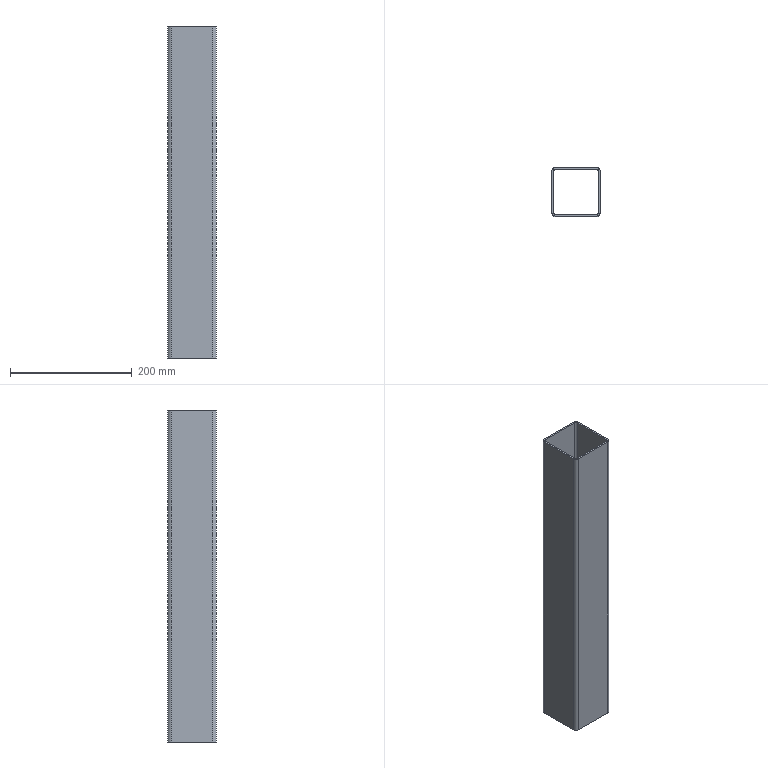Part | STEP file | SN10_008_006-01_TUBO_QUADRADO | 1 solid | 18 faces | box 80 x 80 x 546 mm | volume 491849 mm3 | plane 10 | cylinder 8 | commonest cylinder face diameters 6 x4 12 x4
STEP:
#1=CARTESIAN_POINT('',(0.,0.,0.));
#2=DIRECTION('',(0.,0.,1.));
#3=DIRECTION('',(1.,0.,0.));
#4=AXIS2_PLACEMENT_3D('',#1,#2,#3);
#5=CARTESIAN_POINT('',(323.629,344.,446.));
#6=VERTEX_POINT('',#5);
#7=CARTESIAN_POINT('',(323.629,276.,446.));
#8=VERTEX_POINT('',#7);
#9=CARTESIAN_POINT('',(323.629,344.,446.));
#10=DIRECTION('',(0.,-1.,0.));
#11=VECTOR('',#10,1.);
#12=LINE('',#9,#11);
#13=CARTESIAN_POINT('',(323.629,344.,-115.));
#14=DIRECTION('',(-1.,0.,0.));
#15=DIRECTION('',(0.,0.,1.));
#16=AXIS2_PLACEMENT_3D('',#13,#14,#15);
#17=PLANE('',#16);
#18=CARTESIAN_POINT('',(561.,0.));
#19=DIRECTION('',(0.,-1.));
#20=VECTOR('',#19,1.);
#21=LINE('',#18,#20);
#22=(GEOMETRIC_REPRESENTATION_CONTEXT(2)PARAMETRIC_REPRESENTATION_CONTEXT()REPRESENTATION_CONTEXT('',''));
#23=DEFINITIONAL_REPRESENTATION('',(#21),#22);
#24=PCURVE('',#17,#23);
#25=CARTESIAN_POINT('',(323.629,250.,446.));
#26=DIRECTION('',(0.,0.,-1.));
#27=DIRECTION('',(-1.,0.,0.));
#28=AXIS2_PLACEMENT_3D('',#25,#26,#27);
#29=PLANE('',#28);
#30=CARTESIAN_POINT('',(0.,94.));
#31=DIRECTION('',(0.,-1.));
#32=VECTOR('',#31,1.);
#33=LINE('',#30,#32);
#34=(GEOMETRIC_REPRESENTATION_CONTEXT(2)PARAMETRIC_REPRESENTATION_CONTEXT()REPRESENTATION_CONTEXT('',''));
#35=DEFINITIONAL_REPRESENTATION('',(#33),#34);
#36=PCURVE('',#29,#35);
#37=SURFACE_CURVE('',#12,(#24,#36),.PCURVE_S1.);
#38=EDGE_CURVE('',#6,#8,#37,.T.);
#39=ORIENTED_EDGE('',*,*,#38,.T.);
#40=CARTESIAN_POINT('',(323.629,276.,-100.));
#41=VERTEX_POINT('',#40);
#42=CARTESIAN_POINT('',(323.629,276.,446.));
#43=DIRECTION('',(0.,0.,-1.));
#44=VECTOR('',#43,1.);
#45=LINE('',#42,#44);
#46=CARTESIAN_POINT('',(561.,-68.));
#47=DIRECTION('',(-1.,0.));
#48=VECTOR('',#47,1.);
#49=LINE('',#46,#48);
#50=(GEOMETRIC_REPRESENTATION_CONTEXT(2)PARAMETRIC_REPRESENTATION_CONTEXT()REPRESENTATION_CONTEXT('',''));
#51=DEFINITIONAL_REPRESENTATION('',(#49),#50);
#52=PCURVE('',#17,#51);
#53=CARTESIAN_POINT('',(317.629,276.,176.11));
#54=DIRECTION('',(0.,0.,1.));
#55=DIRECTION('',(0.,-1.,0.));
#56=AXIS2_PLACEMENT_3D('',#53,#54,#55);
#57=CYLINDRICAL_SURFACE('',#56,6.);
#58=CARTESIAN_POINT('',(1.571,269.89));
#59=DIRECTION('',(0.,-1.));
#60=VECTOR('',#59,1.);
#61=LINE('',#58,#60);
#62=(GEOMETRIC_REPRESENTATION_CONTEXT(2)PARAMETRIC_REPRESENTATION_CONTEXT()REPRESENTATION_CONTEXT('',''));
#63=DEFINITIONAL_REPRESENTATION('',(#61),#62);
#64=PCURVE('',#57,#63);
#65=SURFACE_CURVE('',#45,(#52,#64),.PCURVE_S1.);
#66=EDGE_CURVE('',#8,#41,#65,.T.);
#67=ORIENTED_EDGE('',*,*,#66,.T.);
#68=CARTESIAN_POINT('',(323.629,344.,-100.));
#69=VERTEX_POINT('',#68);
#70=CARTESIAN_POINT('',(323.629,344.,-100.));
#71=DIRECTION('',(0.,-1.,0.));
#72=VECTOR('',#71,1.);
#73=LINE('',#70,#72);
#74=CARTESIAN_POINT('',(15.,0.));
#75=DIRECTION('',(0.,-1.));
#76=VECTOR('',#75,1.);
#77=LINE('',#74,#76);
#78=(GEOMETRIC_REPRESENTATION_CONTEXT(2)PARAMETRIC_REPRESENTATION_CONTEXT()REPRESENTATION_CONTEXT('',''));
#79=DEFINITIONAL_REPRESENTATION('',(#77),#78);
#80=PCURVE('',#17,#79);
#81=CARTESIAN_POINT('',(0.,0.,-100.));
#82=DIRECTION('',(0.,0.,1.));
#83=DIRECTION('',(1.,0.,0.));
#84=AXIS2_PLACEMENT_3D('',#81,#82,#83);
#85=PLANE('',#84);
#86=CARTESIAN_POINT('',(323.629,344.));
#87=DIRECTION('',(0.,-1.));
#88=VECTOR('',#87,1.);
#89=LINE('',#86,#88);
#90=(GEOMETRIC_REPRESENTATION_CONTEXT(2)PARAMETRIC_REPRESENTATION_CONTEXT()REPRESENTATION_CONTEXT('',''));
#91=DEFINITIONAL_REPRESENTATION('',(#89),#90);
#92=PCURVE('',#85,#91);
#93=SURFACE_CURVE('',#73,(#80,#92),.PCURVE_S1.);
#94=EDGE_CURVE('',#69,#41,#93,.T.);
#95=ORIENTED_EDGE('',*,*,#94,.F.);
#96=CARTESIAN_POINT('',(323.629,344.,446.));
#97=DIRECTION('',(0.,0.,-1.));
#98=VECTOR('',#97,1.);
#99=LINE('',#96,#98);
#100=CARTESIAN_POINT('',(561.,0.));
#101=DIRECTION('',(-1.,0.));
#102=VECTOR('',#101,1.);
#103=LINE('',#100,#102);
#104=(GEOMETRIC_REPRESENTATION_CONTEXT(2)PARAMETRIC_REPRESENTATION_CONTEXT()REPRESENTATION_CONTEXT('',''));
#105=DEFINITIONAL_REPRESENTATION('',(#103),#104);
#106=PCURVE('',#17,#105);
#107=CARTESIAN_POINT('',(317.629,344.,176.11));
#108=DIRECTION('',(0.,0.,1.));
#109=DIRECTION('',(1.,0.,0.));
#110=AXIS2_PLACEMENT_3D('',#107,#108,#109);
#111=CYLINDRICAL_SURFACE('',#110,6.);
#112=CARTESIAN_POINT('',(0.,269.89));
#113=DIRECTION('',(0.,-1.));
#114=VECTOR('',#113,1.);
#115=LINE('',#112,#114);
#116=(GEOMETRIC_REPRESENTATION_CONTEXT(2)PARAMETRIC_REPRESENTATION_CONTEXT()REPRESENTATION_CONTEXT('',''));
#117=DEFINITIONAL_REPRESENTATION('',(#115),#116);
#118=PCURVE('',#111,#117);
#119=SURFACE_CURVE('',#99,(#106,#118),.PCURVE_S1.);
#120=EDGE_CURVE('',#6,#69,#119,.T.);
#121=ORIENTED_EDGE('',*,*,#120,.F.);
#122=EDGE_LOOP('',(#39,#67,#95,#121));
#123=FACE_BOUND('',#122,.T.);
#124=ADVANCED_FACE('',(#123),#17,.F.);
#125=CARTESIAN_POINT('',(320.629,344.,-100.));
#126=VERTEX_POINT('',#125);
#127=CARTESIAN_POINT('',(320.629,344.,446.));
#128=VERTEX_POINT('',#127);
#129=CARTESIAN_POINT('',(320.629,344.,-100.));
#130=DIRECTION('',(0.,0.,1.));
#131=VECTOR('',#130,1.);
#132=LINE('',#129,#131);
#133=CARTESIAN_POINT('',(317.629,344.,176.11));
#134=DIRECTION('',(0.,0.,1.));
#135=DIRECTION('',(1.,0.,0.));
#136=AXIS2_PLACEMENT_3D('',#133,#134,#135);
#137=CYLINDRICAL_SURFACE('',#136,3.);
#138=CARTESIAN_POINT('',(0.,-276.11));
#139=DIRECTION('',(0.,1.));
#140=VECTOR('',#139,1.);
#141=LINE('',#138,#140);
#142=(GEOMETRIC_REPRESENTATION_CONTEXT(2)PARAMETRIC_REPRESENTATION_CONTEXT()REPRESENTATION_CONTEXT('',''));
#143=DEFINITIONAL_REPRESENTATION('',(#141),#142);
#144=PCURVE('',#137,#143);
#145=CARTESIAN_POINT('',(320.629,344.,-115.));
#146=DIRECTION('',(-1.,0.,0.));
#147=DIRECTION('',(0.,0.,1.));
#148=AXIS2_PLACEMENT_3D('',#145,#146,#147);
#149=PLANE('',#148);
#150=CARTESIAN_POINT('',(15.,0.));
#151=DIRECTION('',(1.,0.));
#152=VECTOR('',#151,1.);
#153=LINE('',#150,#152);
#154=(GEOMETRIC_REPRESENTATION_CONTEXT(2)PARAMETRIC_REPRESENTATION_CONTEXT()REPRESENTATION_CONTEXT('',''));
#155=DEFINITIONAL_REPRESENTATION('',(#153),#154);
#156=PCURVE('',#149,#155);
#157=SURFACE_CURVE('',#132,(#144,#156),.PCURVE_S1.);
#158=EDGE_CURVE('',#126,#128,#157,.T.);
#159=ORIENTED_EDGE('',*,*,#158,.F.);
#160=CARTESIAN_POINT('',(317.629,347.,-100.));
#161=VERTEX_POINT('',#160);
#162=CARTESIAN_POINT('',(317.629,344.,-100.));
#163=DIRECTION('',(0.,0.,1.));
#164=DIRECTION('',(1.,0.,0.));
#165=AXIS2_PLACEMENT_3D('',#162,#163,#164);
#166=CIRCLE('',#165,3.);
#167=CARTESIAN_POINT('',(0.,-276.11));
#168=DIRECTION('',(1.,0.));
#169=VECTOR('',#168,1.);
#170=LINE('',#167,#169);
#171=(GEOMETRIC_REPRESENTATION_CONTEXT(2)PARAMETRIC_REPRESENTATION_CONTEXT()REPRESENTATION_CONTEXT('',''));
#172=DEFINITIONAL_REPRESENTATION('',(#170),#171);
#173=PCURVE('',#137,#172);
#174=CARTESIAN_POINT('',(317.629,344.));
#175=DIRECTION('',(1.,0.));
#176=AXIS2_PLACEMENT_2D('',#174,#175);
#177=CIRCLE('',#176,3.);
#178=(GEOMETRIC_REPRESENTATION_CONTEXT(2)PARAMETRIC_REPRESENTATION_CONTEXT()REPRESENTATION_CONTEXT('',''));
#179=DEFINITIONAL_REPRESENTATION('',(#177),#178);
#180=PCURVE('',#85,#179);
#181=SURFACE_CURVE('',#166,(#173,#180),.PCURVE_S1.);
#182=EDGE_CURVE('',#126,#161,#181,.T.);
#183=ORIENTED_EDGE('',*,*,#182,.T.);
#184=CARTESIAN_POINT('',(317.629,347.,446.));
#185=VERTEX_POINT('',#184);
#186=CARTESIAN_POINT('',(317.629,347.,-100.));
#187=DIRECTION('',(0.,0.,1.));
#188=VECTOR('',#187,1.);
#189=LINE('',#186,#188);
#190=CARTESIAN_POINT('',(1.571,-276.11));
#191=DIRECTION('',(0.,1.));
#192=VECTOR('',#191,1.);
#193=LINE('',#190,#192);
#194=(GEOMETRIC_REPRESENTATION_CONTEXT(2)PARAMETRIC_REPRESENTATION_CONTEXT()REPRESENTATION_CONTEXT('',''));
#195=DEFINITIONAL_REPRESENTATION('',(#193),#194);
#196=PCURVE('',#137,#195);
#197=CARTESIAN_POINT('',(249.629,347.,-115.));
#198=DIRECTION('',(0.,-1.,0.));
#199=DIRECTION('',(0.,0.,-1.));
#200=AXIS2_PLACEMENT_3D('',#197,#198,#199);
#201=PLANE('',#200);
#202=CARTESIAN_POINT('',(-15.,68.));
#203=DIRECTION('',(-1.,0.));
#204=VECTOR('',#203,1.);
#205=LINE('',#202,#204);
#206=(GEOMETRIC_REPRESENTATION_CONTEXT(2)PARAMETRIC_REPRESENTATION_CONTEXT()REPRESENTATION_CONTEXT('',''));
#207=DEFINITIONAL_REPRESENTATION('',(#205),#206);
#208=PCURVE('',#201,#207);
#209=SURFACE_CURVE('',#189,(#196,#208),.PCURVE_S1.);
#210=EDGE_CURVE('',#161,#185,#209,.T.);
#211=ORIENTED_EDGE('',*,*,#210,.T.);
#212=CARTESIAN_POINT('',(317.629,344.,446.));
#213=DIRECTION('',(0.,0.,1.));
#214=DIRECTION('',(1.,0.,0.));
#215=AXIS2_PLACEMENT_3D('',#212,#213,#214);
#216=CIRCLE('',#215,3.);
#217=CARTESIAN_POINT('',(0.,269.89));
#218=DIRECTION('',(1.,0.));
#219=VECTOR('',#218,1.);
#220=LINE('',#217,#219);
#221=(GEOMETRIC_REPRESENTATION_CONTEXT(2)PARAMETRIC_REPRESENTATION_CONTEXT()REPRESENTATION_CONTEXT('',''));
#222=DEFINITIONAL_REPRESENTATION('',(#220),#221);
#223=PCURVE('',#137,#222);
#224=CARTESIAN_POINT('',(3.,94.));
#225=CARTESIAN_POINT('',(3.,99.196));
#226=CARTESIAN_POINT('',(7.5,96.598));
#227=CARTESIAN_POINT('',(12.,94.));
#228=CARTESIAN_POINT('',(7.5,91.402));
#229=CARTESIAN_POINT('',(3.,88.804));
#230=CARTESIAN_POINT('',(3.,94.));
#231=(BOUNDED_CURVE()B_SPLINE_CURVE(2,(#224,#225,#226,#227,#228,#229,#230),.UNSPECIFIED.,.T.,.F.)B_SPLINE_CURVE_WITH_KNOTS((1,2,2,2,2,1),(-2.094,0.,2.094,4.189,6.283,8.378),.UNSPECIFIED.)CURVE()GEOMETRIC_REPRESENTATION_ITEM()RATIONAL_B_SPLINE_CURVE((1.,0.5,1.,0.5,1.,0.5,1.))REPRESENTATION_ITEM(''));
#232=(GEOMETRIC_REPRESENTATION_CONTEXT(2)PARAMETRIC_REPRESENTATION_CONTEXT()REPRESENTATION_CONTEXT('',''));
#233=DEFINITIONAL_REPRESENTATION('',(#231),#232);
#234=PCURVE('',#29,#233);
#235=SURFACE_CURVE('',#216,(#223,#234),.PCURVE_S1.);
#236=EDGE_CURVE('',#128,#185,#235,.T.);
#237=ORIENTED_EDGE('',*,*,#236,.F.);
#238=EDGE_LOOP('',(#159,#183,#211,#237));
#239=FACE_BOUND('',#238,.F.);
#240=ADVANCED_FACE('',(#239),#137,.F.);
#241=ORIENTED_EDGE('',*,*,#158,.F.);
#242=CARTESIAN_POINT('',(320.629,276.,-100.));
#243=VERTEX_POINT('',#242);
#244=CARTESIAN_POINT('',(320.629,344.,-100.));
#245=DIRECTION('',(0.,-1.,0.));
#246=VECTOR('',#245,1.);
#247=LINE('',#244,#246);
#248=CARTESIAN_POINT('',(15.,0.));
#249=DIRECTION('',(0.,-1.));
#250=VECTOR('',#249,1.);
#251=LINE('',#248,#250);
#252=(GEOMETRIC_REPRESENTATION_CONTEXT(2)PARAMETRIC_REPRESENTATION_CONTEXT()REPRESENTATION_CONTEXT('',''));
#253=DEFINITIONAL_REPRESENTATION('',(#251),#252);
#254=PCURVE('',#149,#253);
#255=CARTESIAN_POINT('',(320.629,344.));
#256=DIRECTION('',(0.,-1.));
#257=VECTOR('',#256,1.);
#258=LINE('',#255,#257);
#259=(GEOMETRIC_REPRESENTATION_CONTEXT(2)PARAMETRIC_REPRESENTATION_CONTEXT()REPRESENTATION_CONTEXT('',''));
#260=DEFINITIONAL_REPRESENTATION('',(#258),#259);
#261=PCURVE('',#85,#260);
#262=SURFACE_CURVE('',#247,(#254,#261),.PCURVE_S1.);
#263=EDGE_CURVE('',#126,#243,#262,.T.);
#264=ORIENTED_EDGE('',*,*,#263,.T.);
#265=CARTESIAN_POINT('',(320.629,276.,446.));
#266=VERTEX_POINT('',#265);
#267=CARTESIAN_POINT('',(320.629,276.,446.));
#268=DIRECTION('',(0.,0.,-1.));
#269=VECTOR('',#268,1.);
#270=LINE('',#267,#269);
#271=CARTESIAN_POINT('',(561.,-68.));
#272=DIRECTION('',(-1.,0.));
#273=VECTOR('',#272,1.);
#274=LINE('',#271,#273);
#275=(GEOMETRIC_REPRESENTATION_CONTEXT(2)PARAMETRIC_REPRESENTATION_CONTEXT()REPRESENTATION_CONTEXT('',''));
#276=DEFINITIONAL_REPRESENTATION('',(#274),#275);
#277=PCURVE('',#149,#276);
#278=CARTESIAN_POINT('',(317.629,276.,176.11));
#279=DIRECTION('',(0.,0.,1.));
#280=DIRECTION('',(0.,-1.,0.));
#281=AXIS2_PLACEMENT_3D('',#278,#279,#280);
#282=CYLINDRICAL_SURFACE('',#281,3.);
#283=CARTESIAN_POINT('',(1.571,269.89));
#284=DIRECTION('',(0.,-1.));
#285=VECTOR('',#284,1.);
#286=LINE('',#283,#285);
#287=(GEOMETRIC_REPRESENTATION_CONTEXT(2)PARAMETRIC_REPRESENTATION_CONTEXT()REPRESENTATION_CONTEXT('',''));
#288=DEFINITIONAL_REPRESENTATION('',(#286),#287);
#289=PCURVE('',#282,#288);
#290=SURFACE_CURVE('',#270,(#277,#289),.PCURVE_S1.);
#291=EDGE_CURVE('',#266,#243,#290,.T.);
#292=ORIENTED_EDGE('',*,*,#291,.F.);
#293=CARTESIAN_POINT('',(320.629,344.,446.));
#294=DIRECTION('',(0.,-1.,0.));
#295=VECTOR('',#294,1.);
#296=LINE('',#293,#295);
#297=CARTESIAN_POINT('',(561.,0.));
#298=DIRECTION('',(0.,-1.));
#299=VECTOR('',#298,1.);
#300=LINE('',#297,#299);
#301=(GEOMETRIC_REPRESENTATION_CONTEXT(2)PARAMETRIC_REPRESENTATION_CONTEXT()REPRESENTATION_CONTEXT('',''));
#302=DEFINITIONAL_REPRESENTATION('',(#300),#301);
#303=PCURVE('',#149,#302);
#304=CARTESIAN_POINT('',(3.,94.));
#305=DIRECTION('',(0.,-1.));
#306=VECTOR('',#305,1.);
#307=LINE('',#304,#306);
#308=(GEOMETRIC_REPRESENTATION_CONTEXT(2)PARAMETRIC_REPRESENTATION_CONTEXT()REPRESENTATION_CONTEXT('',''));
#309=DEFINITIONAL_REPRESENTATION('',(#307),#308);
#310=PCURVE('',#29,#309);
#311=SURFACE_CURVE('',#296,(#303,#310),.PCURVE_S1.);
#312=EDGE_CURVE('',#128,#266,#311,.T.);
#313=ORIENTED_EDGE('',*,*,#312,.F.);
#314=EDGE_LOOP('',(#241,#264,#292,#313));
#315=FACE_BOUND('',#314,.T.);
#316=ADVANCED_FACE('',(#315),#149,.T.);
#317=CARTESIAN_POINT('',(317.629,273.,-100.));
#318=VERTEX_POINT('',#317);
#319=CARTESIAN_POINT('',(317.629,273.,446.));
#320=VERTEX_POINT('',#319);
#321=CARTESIAN_POINT('',(317.629,273.,-100.));
#322=DIRECTION('',(0.,0.,1.));
#323=VECTOR('',#322,1.);
#324=LINE('',#321,#323);
#325=CARTESIAN_POINT('',(0.,-276.11));
#326=DIRECTION('',(0.,1.));
#327=VECTOR('',#326,1.);
#328=LINE('',#325,#327);
#329=(GEOMETRIC_REPRESENTATION_CONTEXT(2)PARAMETRIC_REPRESENTATION_CONTEXT()REPRESENTATION_CONTEXT('',''));
#330=DEFINITIONAL_REPRESENTATION('',(#328),#329);
#331=PCURVE('',#282,#330);
#332=CARTESIAN_POINT('',(317.629,273.,-115.));
#333=DIRECTION('',(0.,1.,0.));
#334=DIRECTION('',(0.,0.,1.));
#335=AXIS2_PLACEMENT_3D('',#332,#333,#334);
#336=PLANE('',#335);
#337=CARTESIAN_POINT('',(15.,0.));
#338=DIRECTION('',(1.,0.));
#339=VECTOR('',#338,1.);
#340=LINE('',#337,#339);
#341=(GEOMETRIC_REPRESENTATION_CONTEXT(2)PARAMETRIC_REPRESENTATION_CONTEXT()REPRESENTATION_CONTEXT('',''));
#342=DEFINITIONAL_REPRESENTATION('',(#340),#341);
#343=PCURVE('',#336,#342);
#344=SURFACE_CURVE('',#324,(#331,#343),.PCURVE_S1.);
#345=EDGE_CURVE('',#318,#320,#344,.T.);
#346=ORIENTED_EDGE('',*,*,#345,.F.);
#347=CARTESIAN_POINT('',(317.629,276.,-100.));
#348=DIRECTION('',(0.,0.,1.));
#349=DIRECTION('',(1.,0.,0.));
#350=AXIS2_PLACEMENT_3D('',#347,#348,#349);
#351=CIRCLE('',#350,3.);
#352=CARTESIAN_POINT('',(-4.712,-276.11));
#353=DIRECTION('',(1.,0.));
#354=VECTOR('',#353,1.);
#355=LINE('',#352,#354);
#356=(GEOMETRIC_REPRESENTATION_CONTEXT(2)PARAMETRIC_REPRESENTATION_CONTEXT()REPRESENTATION_CONTEXT('',''));
#357=DEFINITIONAL_REPRESENTATION('',(#355),#356);
#358=PCURVE('',#282,#357);
#359=CARTESIAN_POINT('',(317.629,276.));
#360=DIRECTION('',(1.,0.));
#361=AXIS2_PLACEMENT_2D('',#359,#360);
#362=CIRCLE('',#361,3.);
#363=(GEOMETRIC_REPRESENTATION_CONTEXT(2)PARAMETRIC_REPRESENTATION_CONTEXT()REPRESENTATION_CONTEXT('',''));
#364=DEFINITIONAL_REPRESENTATION('',(#362),#363);
#365=PCURVE('',#85,#364);
#366=SURFACE_CURVE('',#351,(#358,#365),.PCURVE_S1.);
#367=EDGE_CURVE('',#318,#243,#366,.T.);
#368=ORIENTED_EDGE('',*,*,#367,.T.);
#369=ORIENTED_EDGE('',*,*,#291,.F.);
#370=CARTESIAN_POINT('',(317.629,276.,446.));
#371=DIRECTION('',(0.,0.,1.));
#372=DIRECTION('',(1.,0.,0.));
#373=AXIS2_PLACEMENT_3D('',#370,#371,#372);
#374=CIRCLE('',#373,3.);
#375=CARTESIAN_POINT('',(-4.712,269.89));
#376=DIRECTION('',(1.,0.));
#377=VECTOR('',#376,1.);
#378=LINE('',#375,#377);
#379=(GEOMETRIC_REPRESENTATION_CONTEXT(2)PARAMETRIC_REPRESENTATION_CONTEXT()REPRESENTATION_CONTEXT('',''));
#380=DEFINITIONAL_REPRESENTATION('',(#378),#379);
#381=PCURVE('',#282,#380);
#382=CARTESIAN_POINT('',(3.,26.));
#383=CARTESIAN_POINT('',(3.,31.196));
#384=CARTESIAN_POINT('',(7.5,28.598));
#385=CARTESIAN_POINT('',(12.,26.));
#386=CARTESIAN_POINT('',(7.5,23.402));
#387=CARTESIAN_POINT('',(3.,20.804));
#388=CARTESIAN_POINT('',(3.,26.));
#389=(BOUNDED_CURVE()B_SPLINE_CURVE(2,(#382,#383,#384,#385,#386,#387,#388),.UNSPECIFIED.,.T.,.F.)B_SPLINE_CURVE_WITH_KNOTS((1,2,2,2,2,1),(-2.094,0.,2.094,4.189,6.283,8.378),.UNSPECIFIED.)CURVE()GEOMETRIC_REPRESENTATION_ITEM()RATIONAL_B_SPLINE_CURVE((1.,0.5,1.,0.5,1.,0.5,1.))REPRESENTATION_ITEM(''));
#390=(GEOMETRIC_REPRESENTATION_CONTEXT(2)PARAMETRIC_REPRESENTATION_CONTEXT()REPRESENTATION_CONTEXT('',''));
#391=DEFINITIONAL_REPRESENTATION('',(#389),#390);
#392=PCURVE('',#29,#391);
#393=SURFACE_CURVE('',#374,(#381,#392),.PCURVE_S1.);
#394=EDGE_CURVE('',#320,#266,#393,.T.);
#395=ORIENTED_EDGE('',*,*,#394,.F.);
#396=EDGE_LOOP('',(#346,#368,#369,#395));
#397=FACE_BOUND('',#396,.F.);
#398=ADVANCED_FACE('',(#397),#282,.F.);
#399=ORIENTED_EDGE('',*,*,#345,.F.);
#400=CARTESIAN_POINT('',(249.629,273.,-100.));
#401=VERTEX_POINT('',#400);
#402=CARTESIAN_POINT('',(317.629,273.,-100.));
#403=DIRECTION('',(-1.,0.,0.));
#404=VECTOR('',#403,1.);
#405=LINE('',#402,#404);
#406=CARTESIAN_POINT('',(15.,0.));
#407=DIRECTION('',(0.,-1.));
#408=VECTOR('',#407,1.);
#409=LINE('',#406,#408);
#410=(GEOMETRIC_REPRESENTATION_CONTEXT(2)PARAMETRIC_REPRESENTATION_CONTEXT()REPRESENTATION_CONTEXT('',''));
#411=DEFINITIONAL_REPRESENTATION('',(#409),#410);
#412=PCURVE('',#336,#411);
#413=CARTESIAN_POINT('',(317.629,273.));
#414=DIRECTION('',(-1.,0.));
#415=VECTOR('',#414,1.);
#416=LINE('',#413,#415);
#417=(GEOMETRIC_REPRESENTATION_CONTEXT(2)PARAMETRIC_REPRESENTATION_CONTEXT()REPRESENTATION_CONTEXT('',''));
#418=DEFINITIONAL_REPRESENTATION('',(#416),#417);
#419=PCURVE('',#85,#418);
#420=SURFACE_CURVE('',#405,(#412,#419),.PCURVE_S1.);
#421=EDGE_CURVE('',#318,#401,#420,.T.);
#422=ORIENTED_EDGE('',*,*,#421,.T.);
#423=CARTESIAN_POINT('',(249.629,273.,446.));
#424=VERTEX_POINT('',#423);
#425=CARTESIAN_POINT('',(249.629,273.,446.));
#426=DIRECTION('',(0.,0.,-1.));
#427=VECTOR('',#426,1.);
#428=LINE('',#425,#427);
#429=CARTESIAN_POINT('',(561.,-68.));
#430=DIRECTION('',(-1.,0.));
#431=VECTOR('',#430,1.);
#432=LINE('',#429,#431);
#433=(GEOMETRIC_REPRESENTATION_CONTEXT(2)PARAMETRIC_REPRESENTATION_CONTEXT()REPRESENTATION_CONTEXT('',''));
#434=DEFINITIONAL_REPRESENTATION('',(#432),#433);
#435=PCURVE('',#336,#434);
#436=CARTESIAN_POINT('',(249.629,276.,176.11));
#437=DIRECTION('',(0.,0.,1.));
#438=DIRECTION('',(-1.,0.,0.));
#439=AXIS2_PLACEMENT_3D('',#436,#437,#438);
#440=CYLINDRICAL_SURFACE('',#439,3.);
#441=CARTESIAN_POINT('',(1.571,269.89));
#442=DIRECTION('',(0.,-1.));
#443=VECTOR('',#442,1.);
#444=LINE('',#441,#443);
#445=(GEOMETRIC_REPRESENTATION_CONTEXT(2)PARAMETRIC_REPRESENTATION_CONTEXT()REPRESENTATION_CONTEXT('',''));
#446=DEFINITIONAL_REPRESENTATION('',(#444),#445);
#447=PCURVE('',#440,#446);
#448=SURFACE_CURVE('',#428,(#435,#447),.PCURVE_S1.);
#449=EDGE_CURVE('',#424,#401,#448,.T.);
#450=ORIENTED_EDGE('',*,*,#449,.F.);
#451=CARTESIAN_POINT('',(317.629,273.,446.));
#452=DIRECTION('',(-1.,0.,0.));
#453=VECTOR('',#452,1.);
#454=LINE('',#451,#453);
#455=CARTESIAN_POINT('',(561.,0.));
#456=DIRECTION('',(0.,-1.));
#457=VECTOR('',#456,1.);
#458=LINE('',#455,#457);
#459=(GEOMETRIC_REPRESENTATION_CONTEXT(2)PARAMETRIC_REPRESENTATION_CONTEXT()REPRESENTATION_CONTEXT('',''));
#460=DEFINITIONAL_REPRESENTATION('',(#458),#459);
#461=PCURVE('',#336,#460);
#462=CARTESIAN_POINT('',(6.,23.));
#463=DIRECTION('',(1.,0.));
#464=VECTOR('',#463,1.);
#465=LINE('',#462,#464);
#466=(GEOMETRIC_REPRESENTATION_CONTEXT(2)PARAMETRIC_REPRESENTATION_CONTEXT()REPRESENTATION_CONTEXT('',''));
#467=DEFINITIONAL_REPRESENTATION('',(#465),#466);
#468=PCURVE('',#29,#467);
#469=SURFACE_CURVE('',#454,(#461,#468),.PCURVE_S1.);
#470=EDGE_CURVE('',#320,#424,#469,.T.);
#471=ORIENTED_EDGE('',*,*,#470,.F.);
#472=EDGE_LOOP('',(#399,#422,#450,#471));
#473=FACE_BOUND('',#472,.T.);
#474=ADVANCED_FACE('',(#473),#336,.T.);
#475=CARTESIAN_POINT('',(246.629,276.,-100.));
#476=VERTEX_POINT('',#475);
#477=CARTESIAN_POINT('',(246.629,276.,446.));
#478=VERTEX_POINT('',#477);
#479=CARTESIAN_POINT('',(246.629,276.,-100.));
#480=DIRECTION('',(0.,0.,1.));
#481=VECTOR('',#480,1.);
#482=LINE('',#479,#481);
#483=CARTESIAN_POINT('',(0.,-276.11));
#484=DIRECTION('',(0.,1.));
#485=VECTOR('',#484,1.);
#486=LINE('',#483,#485);
#487=(GEOMETRIC_REPRESENTATION_CONTEXT(2)PARAMETRIC_REPRESENTATION_CONTEXT()REPRESENTATION_CONTEXT('',''));
#488=DEFINITIONAL_REPRESENTATION('',(#486),#487);
#489=PCURVE('',#440,#488);
#490=CARTESIAN_POINT('',(246.629,276.,-115.));
#491=DIRECTION('',(1.,0.,0.));
#492=DIRECTION('',(0.,0.,-1.));
#493=AXIS2_PLACEMENT_3D('',#490,#491,#492);
#494=PLANE('',#493);
#495=CARTESIAN_POINT('',(-15.,0.));
#496=DIRECTION('',(-1.,0.));
#497=VECTOR('',#496,1.);
#498=LINE('',#495,#497);
#499=(GEOMETRIC_REPRESENTATION_CONTEXT(2)PARAMETRIC_REPRESENTATION_CONTEXT()REPRESENTATION_CONTEXT('',''));
#500=DEFINITIONAL_REPRESENTATION('',(#498),#499);
#501=PCURVE('',#494,#500);
#502=SURFACE_CURVE('',#482,(#489,#501),.PCURVE_S1.);
#503=EDGE_CURVE('',#476,#478,#502,.T.);
#504=ORIENTED_EDGE('',*,*,#503,.F.);
#505=CARTESIAN_POINT('',(249.629,276.,-100.));
#506=DIRECTION('',(0.,0.,1.));
#507=DIRECTION('',(1.,0.,0.));
#508=AXIS2_PLACEMENT_3D('',#505,#506,#507);
#509=CIRCLE('',#508,3.);
#510=CARTESIAN_POINT('',(-3.142,-276.11));
#511=DIRECTION('',(1.,0.));
#512=VECTOR('',#511,1.);
#513=LINE('',#510,#512);
#514=(GEOMETRIC_REPRESENTATION_CONTEXT(2)PARAMETRIC_REPRESENTATION_CONTEXT()REPRESENTATION_CONTEXT('',''));
#515=DEFINITIONAL_REPRESENTATION('',(#513),#514);
#516=PCURVE('',#440,#515);
#517=CARTESIAN_POINT('',(249.629,276.));
#518=DIRECTION('',(1.,0.));
#519=AXIS2_PLACEMENT_2D('',#517,#518);
#520=CIRCLE('',#519,3.);
#521=(GEOMETRIC_REPRESENTATION_CONTEXT(2)PARAMETRIC_REPRESENTATION_CONTEXT()REPRESENTATION_CONTEXT('',''));
#522=DEFINITIONAL_REPRESENTATION('',(#520),#521);
#523=PCURVE('',#85,#522);
#524=SURFACE_CURVE('',#509,(#516,#523),.PCURVE_S1.);
#525=EDGE_CURVE('',#476,#401,#524,.T.);
#526=ORIENTED_EDGE('',*,*,#525,.T.);
#527=ORIENTED_EDGE('',*,*,#449,.F.);
#528=CARTESIAN_POINT('',(249.629,276.,446.));
#529=DIRECTION('',(0.,0.,1.));
#530=DIRECTION('',(1.,0.,0.));
#531=AXIS2_PLACEMENT_3D('',#528,#529,#530);
#532=CIRCLE('',#531,3.);
#533=CARTESIAN_POINT('',(-3.142,269.89));
#534=DIRECTION('',(1.,0.));
#535=VECTOR('',#534,1.);
#536=LINE('',#533,#535);
#537=(GEOMETRIC_REPRESENTATION_CONTEXT(2)PARAMETRIC_REPRESENTATION_CONTEXT()REPRESENTATION_CONTEXT('',''));
#538=DEFINITIONAL_REPRESENTATION('',(#536),#537);
#539=PCURVE('',#440,#538);
#540=CARTESIAN_POINT('',(71.,26.));
#541=CARTESIAN_POINT('',(71.,31.196));
#542=CARTESIAN_POINT('',(75.5,28.598));
#543=CARTESIAN_POINT('',(80.,26.));
#544=CARTESIAN_POINT('',(75.5,23.402));
#545=CARTESIAN_POINT('',(71.,20.804));
#546=CARTESIAN_POINT('',(71.,26.));
#547=(BOUNDED_CURVE()B_SPLINE_CURVE(2,(#540,#541,#542,#543,#544,#545,#546),.UNSPECIFIED.,.T.,.F.)B_SPLINE_CURVE_WITH_KNOTS((1,2,2,2,2,1),(-2.094,0.,2.094,4.189,6.283,8.378),.UNSPECIFIED.)CURVE()GEOMETRIC_REPRESENTATION_ITEM()RATIONAL_B_SPLINE_CURVE((1.,0.5,1.,0.5,1.,0.5,1.))REPRESENTATION_ITEM(''));
#548=(GEOMETRIC_REPRESENTATION_CONTEXT(2)PARAMETRIC_REPRESENTATION_CONTEXT()REPRESENTATION_CONTEXT('',''));
#549=DEFINITIONAL_REPRESENTATION('',(#547),#548);
#550=PCURVE('',#29,#549);
#551=SURFACE_CURVE('',#532,(#539,#550),.PCURVE_S1.);
#552=EDGE_CURVE('',#478,#424,#551,.T.);
#553=ORIENTED_EDGE('',*,*,#552,.F.);
#554=EDGE_LOOP('',(#504,#526,#527,#553));
#555=FACE_BOUND('',#554,.F.);
#556=ADVANCED_FACE('',(#555),#440,.F.);
#557=ORIENTED_EDGE('',*,*,#503,.F.);
#558=CARTESIAN_POINT('',(246.629,344.,-100.));
#559=VERTEX_POINT('',#558);
#560=CARTESIAN_POINT('',(246.629,276.,-100.));
#561=DIRECTION('',(0.,1.,0.));
#562=VECTOR('',#561,1.);
#563=LINE('',#560,#562);
#564=CARTESIAN_POINT('',(-15.,0.));
#565=DIRECTION('',(0.,1.));
#566=VECTOR('',#565,1.);
#567=LINE('',#564,#566);
#568=(GEOMETRIC_REPRESENTATION_CONTEXT(2)PARAMETRIC_REPRESENTATION_CONTEXT()REPRESENTATION_CONTEXT('',''));
#569=DEFINITIONAL_REPRESENTATION('',(#567),#568);
#570=PCURVE('',#494,#569);
#571=CARTESIAN_POINT('',(246.629,276.));
#572=DIRECTION('',(0.,1.));
#573=VECTOR('',#572,1.);
#574=LINE('',#571,#573);
#575=(GEOMETRIC_REPRESENTATION_CONTEXT(2)PARAMETRIC_REPRESENTATION_CONTEXT()REPRESENTATION_CONTEXT('',''));
#576=DEFINITIONAL_REPRESENTATION('',(#574),#575);
#577=PCURVE('',#85,#576);
#578=SURFACE_CURVE('',#563,(#570,#577),.PCURVE_S1.);
#579=EDGE_CURVE('',#476,#559,#578,.T.);
#580=ORIENTED_EDGE('',*,*,#579,.T.);
#581=CARTESIAN_POINT('',(246.629,344.,446.));
#582=VERTEX_POINT('',#581);
#583=CARTESIAN_POINT('',(246.629,344.,446.));
#584=DIRECTION('',(0.,0.,-1.));
#585=VECTOR('',#584,1.);
#586=LINE('',#583,#585);
#587=CARTESIAN_POINT('',(-561.,68.));
#588=DIRECTION('',(1.,0.));
#589=VECTOR('',#588,1.);
#590=LINE('',#587,#589);
#591=(GEOMETRIC_REPRESENTATION_CONTEXT(2)PARAMETRIC_REPRESENTATION_CONTEXT()REPRESENTATION_CONTEXT('',''));
#592=DEFINITIONAL_REPRESENTATION('',(#590),#591);
#593=PCURVE('',#494,#592);
#594=CARTESIAN_POINT('',(249.629,344.,176.11));
#595=DIRECTION('',(0.,0.,1.));
#596=DIRECTION('',(0.,1.,0.));
#597=AXIS2_PLACEMENT_3D('',#594,#595,#596);
#598=CYLINDRICAL_SURFACE('',#597,3.);
#599=CARTESIAN_POINT('',(1.571,269.89));
#600=DIRECTION('',(0.,-1.));
#601=VECTOR('',#600,1.);
#602=LINE('',#599,#601);
#603=(GEOMETRIC_REPRESENTATION_CONTEXT(2)PARAMETRIC_REPRESENTATION_CONTEXT()REPRESENTATION_CONTEXT('',''));
#604=DEFINITIONAL_REPRESENTATION('',(#602),#603);
#605=PCURVE('',#598,#604);
#606=SURFACE_CURVE('',#586,(#593,#605),.PCURVE_S1.);
#607=EDGE_CURVE('',#582,#559,#606,.T.);
#608=ORIENTED_EDGE('',*,*,#607,.F.);
#609=CARTESIAN_POINT('',(246.629,276.,446.));
#610=DIRECTION('',(0.,1.,0.));
#611=VECTOR('',#610,1.);
#612=LINE('',#609,#611);
#613=CARTESIAN_POINT('',(-561.,0.));
#614=DIRECTION('',(0.,1.));
#615=VECTOR('',#614,1.);
#616=LINE('',#613,#615);
#617=(GEOMETRIC_REPRESENTATION_CONTEXT(2)PARAMETRIC_REPRESENTATION_CONTEXT()REPRESENTATION_CONTEXT('',''));
#618=DEFINITIONAL_REPRESENTATION('',(#616),#617);
#619=PCURVE('',#494,#618);
#620=CARTESIAN_POINT('',(77.,26.));
#621=DIRECTION('',(0.,1.));
#622=VECTOR('',#621,1.);
#623=LINE('',#620,#622);
#624=(GEOMETRIC_REPRESENTATION_CONTEXT(2)PARAMETRIC_REPRESENTATION_CONTEXT()REPRESENTATION_CONTEXT('',''));
#625=DEFINITIONAL_REPRESENTATION('',(#623),#624);
#626=PCURVE('',#29,#625);
#627=SURFACE_CURVE('',#612,(#619,#626),.PCURVE_S1.);
#628=EDGE_CURVE('',#478,#582,#627,.T.);
#629=ORIENTED_EDGE('',*,*,#628,.F.);
#630=EDGE_LOOP('',(#557,#580,#608,#629));
#631=FACE_BOUND('',#630,.T.);
#632=ADVANCED_FACE('',(#631),#494,.T.);
#633=CARTESIAN_POINT('',(249.629,347.,-100.));
#634=VERTEX_POINT('',#633);
#635=CARTESIAN_POINT('',(249.629,347.,446.));
#636=VERTEX_POINT('',#635);
#637=CARTESIAN_POINT('',(249.629,347.,-100.));
#638=DIRECTION('',(0.,0.,1.));
#639=VECTOR('',#638,1.);
#640=LINE('',#637,#639);
#641=CARTESIAN_POINT('',(0.,-276.11));
#642=DIRECTION('',(0.,1.));
#643=VECTOR('',#642,1.);
#644=LINE('',#641,#643);
#645=(GEOMETRIC_REPRESENTATION_CONTEXT(2)PARAMETRIC_REPRESENTATION_CONTEXT()REPRESENTATION_CONTEXT('',''));
#646=DEFINITIONAL_REPRESENTATION('',(#644),#645);
#647=PCURVE('',#598,#646);
#648=CARTESIAN_POINT('',(-15.,0.));
#649=DIRECTION('',(-1.,0.));
#650=VECTOR('',#649,1.);
#651=LINE('',#648,#650);
#652=(GEOMETRIC_REPRESENTATION_CONTEXT(2)PARAMETRIC_REPRESENTATION_CONTEXT()REPRESENTATION_CONTEXT('',''));
#653=DEFINITIONAL_REPRESENTATION('',(#651),#652);
#654=PCURVE('',#201,#653);
#655=SURFACE_CURVE('',#640,(#647,#654),.PCURVE_S1.);
#656=EDGE_CURVE('',#634,#636,#655,.T.);
#657=ORIENTED_EDGE('',*,*,#656,.F.);
#658=CARTESIAN_POINT('',(249.629,344.,-100.));
#659=DIRECTION('',(0.,0.,1.));
#660=DIRECTION('',(1.,0.,0.));
#661=AXIS2_PLACEMENT_3D('',#658,#659,#660);
#662=CIRCLE('',#661,3.);
#663=CARTESIAN_POINT('',(-1.571,-276.11));
#664=DIRECTION('',(1.,0.));
#665=VECTOR('',#664,1.);
#666=LINE('',#663,#665);
#667=(GEOMETRIC_REPRESENTATION_CONTEXT(2)PARAMETRIC_REPRESENTATION_CONTEXT()REPRESENTATION_CONTEXT('',''));
#668=DEFINITIONAL_REPRESENTATION('',(#666),#667);
#669=PCURVE('',#598,#668);
#670=CARTESIAN_POINT('',(249.629,344.));
#671=DIRECTION('',(1.,0.));
#672=AXIS2_PLACEMENT_2D('',#670,#671);
#673=CIRCLE('',#672,3.);
#674=(GEOMETRIC_REPRESENTATION_CONTEXT(2)PARAMETRIC_REPRESENTATION_CONTEXT()REPRESENTATION_CONTEXT('',''));
#675=DEFINITIONAL_REPRESENTATION('',(#673),#674);
#676=PCURVE('',#85,#675);
#677=SURFACE_CURVE('',#662,(#669,#676),.PCURVE_S1.);
#678=EDGE_CURVE('',#634,#559,#677,.T.);
#679=ORIENTED_EDGE('',*,*,#678,.T.);
#680=ORIENTED_EDGE('',*,*,#607,.F.);
#681=CARTESIAN_POINT('',(249.629,344.,446.));
#682=DIRECTION('',(0.,0.,1.));
#683=DIRECTION('',(1.,0.,0.));
#684=AXIS2_PLACEMENT_3D('',#681,#682,#683);
#685=CIRCLE('',#684,3.);
#686=CARTESIAN_POINT('',(-1.571,269.89));
#687=DIRECTION('',(1.,0.));
#688=VECTOR('',#687,1.);
#689=LINE('',#686,#688);
#690=(GEOMETRIC_REPRESENTATION_CONTEXT(2)PARAMETRIC_REPRESENTATION_CONTEXT()REPRESENTATION_CONTEXT('',''));
#691=DEFINITIONAL_REPRESENTATION('',(#689),#690);
#692=PCURVE('',#598,#691);
#693=CARTESIAN_POINT('',(71.,94.));
#694=CARTESIAN_POINT('',(71.,99.196));
#695=CARTESIAN_POINT('',(75.5,96.598));
#696=CARTESIAN_POINT('',(80.,94.));
#697=CARTESIAN_POINT('',(75.5,91.402));
#698=CARTESIAN_POINT('',(71.,88.804));
#699=CARTESIAN_POINT('',(71.,94.));
#700=(BOUNDED_CURVE()B_SPLINE_CURVE(2,(#693,#694,#695,#696,#697,#698,#699),.UNSPECIFIED.,.T.,.F.)B_SPLINE_CURVE_WITH_KNOTS((1,2,2,2,2,1),(-2.094,0.,2.094,4.189,6.283,8.378),.UNSPECIFIED.)CURVE()GEOMETRIC_REPRESENTATION_ITEM()RATIONAL_B_SPLINE_CURVE((1.,0.5,1.,0.5,1.,0.5,1.))REPRESENTATION_ITEM(''));
#701=(GEOMETRIC_REPRESENTATION_CONTEXT(2)PARAMETRIC_REPRESENTATION_CONTEXT()REPRESENTATION_CONTEXT('',''));
#702=DEFINITIONAL_REPRESENTATION('',(#700),#701);
#703=PCURVE('',#29,#702);
#704=SURFACE_CURVE('',#685,(#692,#703),.PCURVE_S1.);
#705=EDGE_CURVE('',#636,#582,#704,.T.);
#706=ORIENTED_EDGE('',*,*,#705,.F.);
#707=EDGE_LOOP('',(#657,#679,#680,#706));
#708=FACE_BOUND('',#707,.F.);
#709=ADVANCED_FACE('',(#708),#598,.F.);
#710=ORIENTED_EDGE('',*,*,#656,.F.);
#711=CARTESIAN_POINT('',(249.629,347.,-100.));
#712=DIRECTION('',(1.,0.,0.));
#713=VECTOR('',#712,1.);
#714=LINE('',#711,#713);
#715=CARTESIAN_POINT('',(-15.,0.));
#716=DIRECTION('',(0.,1.));
#717=VECTOR('',#716,1.);
#718=LINE('',#715,#717);
#719=(GEOMETRIC_REPRESENTATION_CONTEXT(2)PARAMETRIC_REPRESENTATION_CONTEXT()REPRESENTATION_CONTEXT('',''));
#720=DEFINITIONAL_REPRESENTATION('',(#718),#719);
#721=PCURVE('',#201,#720);
#722=CARTESIAN_POINT('',(249.629,347.));
#723=DIRECTION('',(1.,0.));
#724=VECTOR('',#723,1.);
#725=LINE('',#722,#724);
#726=(GEOMETRIC_REPRESENTATION_CONTEXT(2)PARAMETRIC_REPRESENTATION_CONTEXT()REPRESENTATION_CONTEXT('',''));
#727=DEFINITIONAL_REPRESENTATION('',(#725),#726);
#728=PCURVE('',#85,#727);
#729=SURFACE_CURVE('',#714,(#721,#728),.PCURVE_S1.);
#730=EDGE_CURVE('',#634,#161,#729,.T.);
#731=ORIENTED_EDGE('',*,*,#730,.T.);
#732=ORIENTED_EDGE('',*,*,#210,.T.);
#733=CARTESIAN_POINT('',(249.629,347.,446.));
#734=DIRECTION('',(1.,0.,0.));
#735=VECTOR('',#734,1.);
#736=LINE('',#733,#735);
#737=CARTESIAN_POINT('',(-561.,0.));
#738=DIRECTION('',(0.,1.));
#739=VECTOR('',#738,1.);
#740=LINE('',#737,#739);
#741=(GEOMETRIC_REPRESENTATION_CONTEXT(2)PARAMETRIC_REPRESENTATION_CONTEXT()REPRESENTATION_CONTEXT('',''));
#742=DEFINITIONAL_REPRESENTATION('',(#740),#741);
#743=PCURVE('',#201,#742);
#744=CARTESIAN_POINT('',(74.,97.));
#745=DIRECTION('',(-1.,0.));
#746=VECTOR('',#745,1.);
#747=LINE('',#744,#746);
#748=(GEOMETRIC_REPRESENTATION_CONTEXT(2)PARAMETRIC_REPRESENTATION_CONTEXT()REPRESENTATION_CONTEXT('',''));
#749=DEFINITIONAL_REPRESENTATION('',(#747),#748);
#750=PCURVE('',#29,#749);
#751=SURFACE_CURVE('',#736,(#743,#750),.PCURVE_S1.);
#752=EDGE_CURVE('',#636,#185,#751,.T.);
#753=ORIENTED_EDGE('',*,*,#752,.F.);
#754=EDGE_LOOP('',(#710,#731,#732,#753));
#755=FACE_BOUND('',#754,.T.);
#756=ADVANCED_FACE('',(#755),#201,.T.);
#757=CARTESIAN_POINT('',(249.629,350.,-100.));
#758=VERTEX_POINT('',#757);
#759=CARTESIAN_POINT('',(249.629,350.,446.));
#760=VERTEX_POINT('',#759);
#761=CARTESIAN_POINT('',(249.629,350.,-100.));
#762=DIRECTION('',(0.,0.,1.));
#763=VECTOR('',#762,1.);
#764=LINE('',#761,#763);
#765=CARTESIAN_POINT('',(249.629,344.,176.11));
#766=DIRECTION('',(0.,0.,1.));
#767=DIRECTION('',(0.,1.,0.));
#768=AXIS2_PLACEMENT_3D('',#765,#766,#767);
#769=CYLINDRICAL_SURFACE('',#768,6.);
#770=CARTESIAN_POINT('',(0.,-276.11));
#771=DIRECTION('',(0.,1.));
#772=VECTOR('',#771,1.);
#773=LINE('',#770,#772);
#774=(GEOMETRIC_REPRESENTATION_CONTEXT(2)PARAMETRIC_REPRESENTATION_CONTEXT()REPRESENTATION_CONTEXT('',''));
#775=DEFINITIONAL_REPRESENTATION('',(#773),#774);
#776=PCURVE('',#769,#775);
#777=CARTESIAN_POINT('',(249.629,350.,-115.));
#778=DIRECTION('',(0.,-1.,0.));
#779=DIRECTION('',(0.,0.,-1.));
#780=AXIS2_PLACEMENT_3D('',#777,#778,#779);
#781=PLANE('',#780);
#782=CARTESIAN_POINT('',(-15.,0.));
#783=DIRECTION('',(-1.,0.));
#784=VECTOR('',#783,1.);
#785=LINE('',#782,#784);
#786=(GEOMETRIC_REPRESENTATION_CONTEXT(2)PARAMETRIC_REPRESENTATION_CONTEXT()REPRESENTATION_CONTEXT('',''));
#787=DEFINITIONAL_REPRESENTATION('',(#785),#786);
#788=PCURVE('',#781,#787);
#789=SURFACE_CURVE('',#764,(#776,#788),.PCURVE_S1.);
#790=EDGE_CURVE('',#758,#760,#789,.T.);
#791=ORIENTED_EDGE('',*,*,#790,.F.);
#792=CARTESIAN_POINT('',(243.629,344.,-100.));
#793=VERTEX_POINT('',#792);
#794=CARTESIAN_POINT('',(249.629,344.,-100.));
#795=DIRECTION('',(0.,0.,1.));
#796=DIRECTION('',(1.,0.,0.));
#797=AXIS2_PLACEMENT_3D('',#794,#795,#796);
#798=CIRCLE('',#797,6.);
#799=CARTESIAN_POINT('',(-1.571,-276.11));
#800=DIRECTION('',(1.,0.));
#801=VECTOR('',#800,1.);
#802=LINE('',#799,#801);
#803=(GEOMETRIC_REPRESENTATION_CONTEXT(2)PARAMETRIC_REPRESENTATION_CONTEXT()REPRESENTATION_CONTEXT('',''));
#804=DEFINITIONAL_REPRESENTATION('',(#802),#803);
#805=PCURVE('',#769,#804);
#806=CARTESIAN_POINT('',(249.629,344.));
#807=DIRECTION('',(1.,0.));
#808=AXIS2_PLACEMENT_2D('',#806,#807);
#809=CIRCLE('',#808,6.);
#810=(GEOMETRIC_REPRESENTATION_CONTEXT(2)PARAMETRIC_REPRESENTATION_CONTEXT()REPRESENTATION_CONTEXT('',''));
#811=DEFINITIONAL_REPRESENTATION('',(#809),#810);
#812=PCURVE('',#85,#811);
#813=SURFACE_CURVE('',#798,(#805,#812),.PCURVE_S1.);
#814=EDGE_CURVE('',#758,#793,#813,.T.);
#815=ORIENTED_EDGE('',*,*,#814,.T.);
#816=CARTESIAN_POINT('',(243.629,344.,446.));
#817=VERTEX_POINT('',#816);
#818=CARTESIAN_POINT('',(243.629,344.,-100.));
#819=DIRECTION('',(0.,0.,1.));
#820=VECTOR('',#819,1.);
#821=LINE('',#818,#820);
#822=CARTESIAN_POINT('',(1.571,-276.11));
#823=DIRECTION('',(0.,1.));
#824=VECTOR('',#823,1.);
#825=LINE('',#822,#824);
#826=(GEOMETRIC_REPRESENTATION_CONTEXT(2)PARAMETRIC_REPRESENTATION_CONTEXT()REPRESENTATION_CONTEXT('',''));
#827=DEFINITIONAL_REPRESENTATION('',(#825),#826);
#828=PCURVE('',#769,#827);
#829=CARTESIAN_POINT('',(243.629,276.,-115.));
#830=DIRECTION('',(1.,0.,0.));
#831=DIRECTION('',(0.,0.,-1.));
#832=AXIS2_PLACEMENT_3D('',#829,#830,#831);
#833=PLANE('',#832);
#834=CARTESIAN_POINT('',(-15.,68.));
#835=DIRECTION('',(-1.,0.));
#836=VECTOR('',#835,1.);
#837=LINE('',#834,#836);
#838=(GEOMETRIC_REPRESENTATION_CONTEXT(2)PARAMETRIC_REPRESENTATION_CONTEXT()REPRESENTATION_CONTEXT('',''));
#839=DEFINITIONAL_REPRESENTATION('',(#837),#838);
#840=PCURVE('',#833,#839);
#841=SURFACE_CURVE('',#821,(#828,#840),.PCURVE_S1.);
#842=EDGE_CURVE('',#793,#817,#841,.T.);
#843=ORIENTED_EDGE('',*,*,#842,.T.);
#844=CARTESIAN_POINT('',(249.629,344.,446.));
#845=DIRECTION('',(0.,0.,1.));
#846=DIRECTION('',(1.,0.,0.));
#847=AXIS2_PLACEMENT_3D('',#844,#845,#846);
#848=CIRCLE('',#847,6.);
#849=CARTESIAN_POINT('',(-1.571,269.89));
#850=DIRECTION('',(1.,0.));
#851=VECTOR('',#850,1.);
#852=LINE('',#849,#851);
#853=(GEOMETRIC_REPRESENTATION_CONTEXT(2)PARAMETRIC_REPRESENTATION_CONTEXT()REPRESENTATION_CONTEXT('',''));
#854=DEFINITIONAL_REPRESENTATION('',(#852),#853);
#855=PCURVE('',#769,#854);
#856=CARTESIAN_POINT('',(68.,94.));
#857=CARTESIAN_POINT('',(68.,104.392));
#858=CARTESIAN_POINT('',(77.,99.196));
#859=CARTESIAN_POINT('',(86.,94.));
#860=CARTESIAN_POINT('',(77.,88.804));
#861=CARTESIAN_POINT('',(68.,83.608));
#862=CARTESIAN_POINT('',(68.,94.));
#863=(BOUNDED_CURVE()B_SPLINE_CURVE(2,(#856,#857,#858,#859,#860,#861,#862),.UNSPECIFIED.,.T.,.F.)B_SPLINE_CURVE_WITH_KNOTS((1,2,2,2,2,1),(-2.094,0.,2.094,4.189,6.283,8.378),.UNSPECIFIED.)CURVE()GEOMETRIC_REPRESENTATION_ITEM()RATIONAL_B_SPLINE_CURVE((1.,0.5,1.,0.5,1.,0.5,1.))REPRESENTATION_ITEM(''));
#864=(GEOMETRIC_REPRESENTATION_CONTEXT(2)PARAMETRIC_REPRESENTATION_CONTEXT()REPRESENTATION_CONTEXT('',''));
#865=DEFINITIONAL_REPRESENTATION('',(#863),#864);
#866=PCURVE('',#29,#865);
#867=SURFACE_CURVE('',#848,(#855,#866),.PCURVE_S1.);
#868=EDGE_CURVE('',#760,#817,#867,.T.);
#869=ORIENTED_EDGE('',*,*,#868,.F.);
#870=EDGE_LOOP('',(#791,#815,#843,#869));
#871=FACE_BOUND('',#870,.T.);
#872=ADVANCED_FACE('',(#871),#769,.T.);
#873=CARTESIAN_POINT('',(243.629,276.,446.));
#874=VERTEX_POINT('',#873);
#875=CARTESIAN_POINT('',(243.629,276.,446.));
#876=DIRECTION('',(0.,1.,0.));
#877=VECTOR('',#876,1.);
#878=LINE('',#875,#877);
#879=CARTESIAN_POINT('',(-561.,0.));
#880=DIRECTION('',(0.,1.));
#881=VECTOR('',#880,1.);
#882=LINE('',#879,#881);
#883=(GEOMETRIC_REPRESENTATION_CONTEXT(2)PARAMETRIC_REPRESENTATION_CONTEXT()REPRESENTATION_CONTEXT('',''));
#884=DEFINITIONAL_REPRESENTATION('',(#882),#883);
#885=PCURVE('',#833,#884);
#886=CARTESIAN_POINT('',(80.,26.));
#887=DIRECTION('',(0.,1.));
#888=VECTOR('',#887,1.);
#889=LINE('',#886,#888);
#890=(GEOMETRIC_REPRESENTATION_CONTEXT(2)PARAMETRIC_REPRESENTATION_CONTEXT()REPRESENTATION_CONTEXT('',''));
#891=DEFINITIONAL_REPRESENTATION('',(#889),#890);
#892=PCURVE('',#29,#891);
#893=SURFACE_CURVE('',#878,(#885,#892),.PCURVE_S1.);
#894=EDGE_CURVE('',#874,#817,#893,.T.);
#895=ORIENTED_EDGE('',*,*,#894,.T.);
#896=ORIENTED_EDGE('',*,*,#842,.F.);
#897=CARTESIAN_POINT('',(243.629,276.,-100.));
#898=VERTEX_POINT('',#897);
#899=CARTESIAN_POINT('',(243.629,276.,-100.));
#900=DIRECTION('',(0.,1.,0.));
#901=VECTOR('',#900,1.);
#902=LINE('',#899,#901);
#903=CARTESIAN_POINT('',(-15.,0.));
#904=DIRECTION('',(0.,1.));
#905=VECTOR('',#904,1.);
#906=LINE('',#903,#905);
#907=(GEOMETRIC_REPRESENTATION_CONTEXT(2)PARAMETRIC_REPRESENTATION_CONTEXT()REPRESENTATION_CONTEXT('',''));
#908=DEFINITIONAL_REPRESENTATION('',(#906),#907);
#909=PCURVE('',#833,#908);
#910=CARTESIAN_POINT('',(243.629,276.));
#911=DIRECTION('',(0.,1.));
#912=VECTOR('',#911,1.);
#913=LINE('',#910,#912);
#914=(GEOMETRIC_REPRESENTATION_CONTEXT(2)PARAMETRIC_REPRESENTATION_CONTEXT()REPRESENTATION_CONTEXT('',''));
#915=DEFINITIONAL_REPRESENTATION('',(#913),#914);
#916=PCURVE('',#85,#915);
#917=SURFACE_CURVE('',#902,(#909,#916),.PCURVE_S1.);
#918=EDGE_CURVE('',#898,#793,#917,.T.);
#919=ORIENTED_EDGE('',*,*,#918,.F.);
#920=CARTESIAN_POINT('',(243.629,276.,446.));
#921=DIRECTION('',(0.,0.,-1.));
#922=VECTOR('',#921,1.);
#923=LINE('',#920,#922);
#924=CARTESIAN_POINT('',(-561.,0.));
#925=DIRECTION('',(1.,0.));
#926=VECTOR('',#925,1.);
#927=LINE('',#924,#926);
#928=(GEOMETRIC_REPRESENTATION_CONTEXT(2)PARAMETRIC_REPRESENTATION_CONTEXT()REPRESENTATION_CONTEXT('',''));
#929=DEFINITIONAL_REPRESENTATION('',(#927),#928);
#930=PCURVE('',#833,#929);
#931=CARTESIAN_POINT('',(249.629,276.,176.11));
#932=DIRECTION('',(0.,0.,1.));
#933=DIRECTION('',(-1.,0.,0.));
#934=AXIS2_PLACEMENT_3D('',#931,#932,#933);
#935=CYLINDRICAL_SURFACE('',#934,6.);
#936=CARTESIAN_POINT('',(0.,269.89));
#937=DIRECTION('',(0.,-1.));
#938=VECTOR('',#937,1.);
#939=LINE('',#936,#938);
#940=(GEOMETRIC_REPRESENTATION_CONTEXT(2)PARAMETRIC_REPRESENTATION_CONTEXT()REPRESENTATION_CONTEXT('',''));
#941=DEFINITIONAL_REPRESENTATION('',(#939),#940);
#942=PCURVE('',#935,#941);
#943=SURFACE_CURVE('',#923,(#930,#942),.PCURVE_S1.);
#944=EDGE_CURVE('',#874,#898,#943,.T.);
#945=ORIENTED_EDGE('',*,*,#944,.F.);
#946=EDGE_LOOP('',(#895,#896,#919,#945));
#947=FACE_BOUND('',#946,.T.);
#948=ADVANCED_FACE('',(#947),#833,.F.);
#949=ORIENTED_EDGE('',*,*,#944,.T.);
#950=CARTESIAN_POINT('',(249.629,270.,-100.));
#951=VERTEX_POINT('',#950);
#952=CARTESIAN_POINT('',(249.629,276.,-100.));
#953=DIRECTION('',(0.,0.,1.));
#954=DIRECTION('',(1.,0.,0.));
#955=AXIS2_PLACEMENT_3D('',#952,#953,#954);
#956=CIRCLE('',#955,6.);
#957=CARTESIAN_POINT('',(-3.142,-276.11));
#958=DIRECTION('',(1.,0.));
#959=VECTOR('',#958,1.);
#960=LINE('',#957,#959);
#961=(GEOMETRIC_REPRESENTATION_CONTEXT(2)PARAMETRIC_REPRESENTATION_CONTEXT()REPRESENTATION_CONTEXT('',''));
#962=DEFINITIONAL_REPRESENTATION('',(#960),#961);
#963=PCURVE('',#935,#962);
#964=CARTESIAN_POINT('',(249.629,276.));
#965=DIRECTION('',(1.,0.));
#966=AXIS2_PLACEMENT_2D('',#964,#965);
#967=CIRCLE('',#966,6.);
#968=(GEOMETRIC_REPRESENTATION_CONTEXT(2)PARAMETRIC_REPRESENTATION_CONTEXT()REPRESENTATION_CONTEXT('',''));
#969=DEFINITIONAL_REPRESENTATION('',(#967),#968);
#970=PCURVE('',#85,#969);
#971=SURFACE_CURVE('',#956,(#963,#970),.PCURVE_S1.);
#972=EDGE_CURVE('',#898,#951,#971,.T.);
#973=ORIENTED_EDGE('',*,*,#972,.T.);
#974=CARTESIAN_POINT('',(249.629,270.,446.));
#975=VERTEX_POINT('',#974);
#976=CARTESIAN_POINT('',(249.629,270.,-100.));
#977=DIRECTION('',(0.,0.,1.));
#978=VECTOR('',#977,1.);
#979=LINE('',#976,#978);
#980=CARTESIAN_POINT('',(1.571,-276.11));
#981=DIRECTION('',(0.,1.));
#982=VECTOR('',#981,1.);
#983=LINE('',#980,#982);
#984=(GEOMETRIC_REPRESENTATION_CONTEXT(2)PARAMETRIC_REPRESENTATION_CONTEXT()REPRESENTATION_CONTEXT('',''));
#985=DEFINITIONAL_REPRESENTATION('',(#983),#984);
#986=PCURVE('',#935,#985);
#987=CARTESIAN_POINT('',(317.629,270.,-115.));
#988=DIRECTION('',(0.,1.,0.));
#989=DIRECTION('',(0.,0.,1.));
#990=AXIS2_PLACEMENT_3D('',#987,#988,#989);
#991=PLANE('',#990);
#992=CARTESIAN_POINT('',(15.,-68.));
#993=DIRECTION('',(1.,0.));
#994=VECTOR('',#993,1.);
#995=LINE('',#992,#994);
#996=(GEOMETRIC_REPRESENTATION_CONTEXT(2)PARAMETRIC_REPRESENTATION_CONTEXT()REPRESENTATION_CONTEXT('',''));
#997=DEFINITIONAL_REPRESENTATION('',(#995),#996);
#998=PCURVE('',#991,#997);
#999=SURFACE_CURVE('',#979,(#986,#998),.PCURVE_S1.);
#1000=EDGE_CURVE('',#951,#975,#999,.T.);
#1001=ORIENTED_EDGE('',*,*,#1000,.T.);
#1002=CARTESIAN_POINT('',(249.629,276.,446.));
#1003=DIRECTION('',(0.,0.,1.));
#1004=DIRECTION('',(1.,0.,0.));
#1005=AXIS2_PLACEMENT_3D('',#1002,#1003,#1004);
#1006=CIRCLE('',#1005,6.);
#1007=CARTESIAN_POINT('',(-3.142,269.89));
#1008=DIRECTION('',(1.,0.));
#1009=VECTOR('',#1008,1.);
#1010=LINE('',#1007,#1009);
#1011=(GEOMETRIC_REPRESENTATION_CONTEXT(2)PARAMETRIC_REPRESENTATION_CONTEXT()REPRESENTATION_CONTEXT('',''));
#1012=DEFINITIONAL_REPRESENTATION('',(#1010),#1011);
#1013=PCURVE('',#935,#1012);
#1014=CARTESIAN_POINT('',(68.,26.));
#1015=CARTESIAN_POINT('',(68.,36.392));
#1016=CARTESIAN_POINT('',(77.,31.196));
#1017=CARTESIAN_POINT('',(86.,26.));
#1018=CARTESIAN_POINT('',(77.,20.804));
#1019=CARTESIAN_POINT('',(68.,15.608));
#1020=CARTESIAN_POINT('',(68.,26.));
#1021=(BOUNDED_CURVE()B_SPLINE_CURVE(2,(#1014,#1015,#1016,#1017,#1018,#1019,#1020),.UNSPECIFIED.,.T.,.F.)B_SPLINE_CURVE_WITH_KNOTS((1,2,2,2,2,1),(-2.094,0.,2.094,4.189,6.283,8.378),.UNSPECIFIED.)CURVE()GEOMETRIC_REPRESENTATION_ITEM()RATIONAL_B_SPLINE_CURVE((1.,0.5,1.,0.5,1.,0.5,1.))REPRESENTATION_ITEM(''));
#1022=(GEOMETRIC_REPRESENTATION_CONTEXT(2)PARAMETRIC_REPRESENTATION_CONTEXT()REPRESENTATION_CONTEXT('',''));
#1023=DEFINITIONAL_REPRESENTATION('',(#1021),#1022);
#1024=PCURVE('',#29,#1023);
#1025=SURFACE_CURVE('',#1006,(#1013,#1024),.PCURVE_S1.);
#1026=EDGE_CURVE('',#874,#975,#1025,.T.);
#1027=ORIENTED_EDGE('',*,*,#1026,.F.);
#1028=EDGE_LOOP('',(#949,#973,#1001,#1027));
#1029=FACE_BOUND('',#1028,.T.);
#1030=ADVANCED_FACE('',(#1029),#935,.T.);
#1031=CARTESIAN_POINT('',(317.629,270.,446.));
#1032=VERTEX_POINT('',#1031);
#1033=CARTESIAN_POINT('',(317.629,270.,446.));
#1034=DIRECTION('',(-1.,0.,0.));
#1035=VECTOR('',#1034,1.);
#1036=LINE('',#1033,#1035);
#1037=CARTESIAN_POINT('',(561.,0.));
#1038=DIRECTION('',(0.,-1.));
#1039=VECTOR('',#1038,1.);
#1040=LINE('',#1037,#1039);
#1041=(GEOMETRIC_REPRESENTATION_CONTEXT(2)PARAMETRIC_REPRESENTATION_CONTEXT()REPRESENTATION_CONTEXT('',''));
#1042=DEFINITIONAL_REPRESENTATION('',(#1040),#1041);
#1043=PCURVE('',#991,#1042);
#1044=CARTESIAN_POINT('',(6.,20.));
#1045=DIRECTION('',(1.,0.));
#1046=VECTOR('',#1045,1.);
#1047=LINE('',#1044,#1046);
#1048=(GEOMETRIC_REPRESENTATION_CONTEXT(2)PARAMETRIC_REPRESENTATION_CONTEXT()REPRESENTATION_CONTEXT('',''));
#1049=DEFINITIONAL_REPRESENTATION('',(#1047),#1048);
#1050=PCURVE('',#29,#1049);
#1051=SURFACE_CURVE('',#1036,(#1043,#1050),.PCURVE_S1.);
#1052=EDGE_CURVE('',#1032,#975,#1051,.T.);
#1053=ORIENTED_EDGE('',*,*,#1052,.T.);
#1054=ORIENTED_EDGE('',*,*,#1000,.F.);
#1055=CARTESIAN_POINT('',(317.629,270.,-100.));
#1056=VERTEX_POINT('',#1055);
#1057=CARTESIAN_POINT('',(317.629,270.,-100.));
#1058=DIRECTION('',(-1.,0.,0.));
#1059=VECTOR('',#1058,1.);
#1060=LINE('',#1057,#1059);
#1061=CARTESIAN_POINT('',(15.,0.));
#1062=DIRECTION('',(0.,-1.));
#1063=VECTOR('',#1062,1.);
#1064=LINE('',#1061,#1063);
#1065=(GEOMETRIC_REPRESENTATION_CONTEXT(2)PARAMETRIC_REPRESENTATION_CONTEXT()REPRESENTATION_CONTEXT('',''));
#1066=DEFINITIONAL_REPRESENTATION('',(#1064),#1065);
#1067=PCURVE('',#991,#1066);
#1068=CARTESIAN_POINT('',(317.629,270.));
#1069=DIRECTION('',(-1.,0.));
#1070=VECTOR('',#1069,1.);
#1071=LINE('',#1068,#1070);
#1072=(GEOMETRIC_REPRESENTATION_CONTEXT(2)PARAMETRIC_REPRESENTATION_CONTEXT()REPRESENTATION_CONTEXT('',''));
#1073=DEFINITIONAL_REPRESENTATION('',(#1071),#1072);
#1074=PCURVE('',#85,#1073);
#1075=SURFACE_CURVE('',#1060,(#1067,#1074),.PCURVE_S1.);
#1076=EDGE_CURVE('',#1056,#951,#1075,.T.);
#1077=ORIENTED_EDGE('',*,*,#1076,.F.);
#1078=CARTESIAN_POINT('',(317.629,270.,446.));
#1079=DIRECTION('',(0.,0.,-1.));
#1080=VECTOR('',#1079,1.);
#1081=LINE('',#1078,#1080);
#1082=CARTESIAN_POINT('',(561.,0.));
#1083=DIRECTION('',(-1.,0.));
#1084=VECTOR('',#1083,1.);
#1085=LINE('',#1082,#1084);
#1086=(GEOMETRIC_REPRESENTATION_CONTEXT(2)PARAMETRIC_REPRESENTATION_CONTEXT()REPRESENTATION_CONTEXT('',''));
#1087=DEFINITIONAL_REPRESENTATION('',(#1085),#1086);
#1088=PCURVE('',#991,#1087);
#1089=CARTESIAN_POINT('',(0.,269.89));
#1090=DIRECTION('',(0.,-1.));
#1091=VECTOR('',#1090,1.);
#1092=LINE('',#1089,#1091);
#1093=(GEOMETRIC_REPRESENTATION_CONTEXT(2)PARAMETRIC_REPRESENTATION_CONTEXT()REPRESENTATION_CONTEXT('',''));
#1094=DEFINITIONAL_REPRESENTATION('',(#1092),#1093);
#1095=PCURVE('',#57,#1094);
#1096=SURFACE_CURVE('',#1081,(#1088,#1095),.PCURVE_S1.);
#1097=EDGE_CURVE('',#1032,#1056,#1096,.T.);
#1098=ORIENTED_EDGE('',*,*,#1097,.F.);
#1099=EDGE_LOOP('',(#1053,#1054,#1077,#1098));
#1100=FACE_BOUND('',#1099,.T.);
#1101=ADVANCED_FACE('',(#1100),#991,.F.);
#1102=CARTESIAN_POINT('',(317.629,350.,446.));
#1103=VERTEX_POINT('',#1102);
#1104=CARTESIAN_POINT('',(249.629,350.,446.));
#1105=DIRECTION('',(1.,0.,0.));
#1106=VECTOR('',#1105,1.);
#1107=LINE('',#1104,#1106);
#1108=CARTESIAN_POINT('',(-561.,0.));
#1109=DIRECTION('',(0.,1.));
#1110=VECTOR('',#1109,1.);
#1111=LINE('',#1108,#1110);
#1112=(GEOMETRIC_REPRESENTATION_CONTEXT(2)PARAMETRIC_REPRESENTATION_CONTEXT()REPRESENTATION_CONTEXT('',''));
#1113=DEFINITIONAL_REPRESENTATION('',(#1111),#1112);
#1114=PCURVE('',#781,#1113);
#1115=CARTESIAN_POINT('',(74.,100.));
#1116=DIRECTION('',(-1.,0.));
#1117=VECTOR('',#1116,1.);
#1118=LINE('',#1115,#1117);
#1119=(GEOMETRIC_REPRESENTATION_CONTEXT(2)PARAMETRIC_REPRESENTATION_CONTEXT()REPRESENTATION_CONTEXT('',''));
#1120=DEFINITIONAL_REPRESENTATION('',(#1118),#1119);
#1121=PCURVE('',#29,#1120);
#1122=SURFACE_CURVE('',#1107,(#1114,#1121),.PCURVE_S1.);
#1123=EDGE_CURVE('',#760,#1103,#1122,.T.);
#1124=ORIENTED_EDGE('',*,*,#1123,.T.);
#1125=CARTESIAN_POINT('',(317.629,350.,-100.));
#1126=VERTEX_POINT('',#1125);
#1127=CARTESIAN_POINT('',(317.629,350.,446.));
#1128=DIRECTION('',(0.,0.,-1.));
#1129=VECTOR('',#1128,1.);
#1130=LINE('',#1127,#1129);
#1131=CARTESIAN_POINT('',(-561.,68.));
#1132=DIRECTION('',(1.,0.));
#1133=VECTOR('',#1132,1.);
#1134=LINE('',#1131,#1133);
#1135=(GEOMETRIC_REPRESENTATION_CONTEXT(2)PARAMETRIC_REPRESENTATION_CONTEXT()REPRESENTATION_CONTEXT('',''));
#1136=DEFINITIONAL_REPRESENTATION('',(#1134),#1135);
#1137=PCURVE('',#781,#1136);
#1138=CARTESIAN_POINT('',(1.571,269.89));
#1139=DIRECTION('',(0.,-1.));
#1140=VECTOR('',#1139,1.);
#1141=LINE('',#1138,#1140);
#1142=(GEOMETRIC_REPRESENTATION_CONTEXT(2)PARAMETRIC_REPRESENTATION_CONTEXT()REPRESENTATION_CONTEXT('',''));
#1143=DEFINITIONAL_REPRESENTATION('',(#1141),#1142);
#1144=PCURVE('',#111,#1143);
#1145=SURFACE_CURVE('',#1130,(#1137,#1144),.PCURVE_S1.);
#1146=EDGE_CURVE('',#1103,#1126,#1145,.T.);
#1147=ORIENTED_EDGE('',*,*,#1146,.T.);
#1148=CARTESIAN_POINT('',(249.629,350.,-100.));
#1149=DIRECTION('',(1.,0.,0.));
#1150=VECTOR('',#1149,1.);
#1151=LINE('',#1148,#1150);
#1152=CARTESIAN_POINT('',(-15.,0.));
#1153=DIRECTION('',(0.,1.));
#1154=VECTOR('',#1153,1.);
#1155=LINE('',#1152,#1154);
#1156=(GEOMETRIC_REPRESENTATION_CONTEXT(2)PARAMETRIC_REPRESENTATION_CONTEXT()REPRESENTATION_CONTEXT('',''));
#1157=DEFINITIONAL_REPRESENTATION('',(#1155),#1156);
#1158=PCURVE('',#781,#1157);
#1159=CARTESIAN_POINT('',(249.629,350.));
#1160=DIRECTION('',(1.,0.));
#1161=VECTOR('',#1160,1.);
#1162=LINE('',#1159,#1161);
#1163=(GEOMETRIC_REPRESENTATION_CONTEXT(2)PARAMETRIC_REPRESENTATION_CONTEXT()REPRESENTATION_CONTEXT('',''));
#1164=DEFINITIONAL_REPRESENTATION('',(#1162),#1163);
#1165=PCURVE('',#85,#1164);
#1166=SURFACE_CURVE('',#1151,(#1158,#1165),.PCURVE_S1.);
#1167=EDGE_CURVE('',#758,#1126,#1166,.T.);
#1168=ORIENTED_EDGE('',*,*,#1167,.F.);
#1169=ORIENTED_EDGE('',*,*,#790,.T.);
#1170=EDGE_LOOP('',(#1124,#1147,#1168,#1169));
#1171=FACE_BOUND('',#1170,.T.);
#1172=ADVANCED_FACE('',(#1171),#781,.F.);
#1173=ORIENTED_EDGE('',*,*,#1097,.T.);
#1174=CARTESIAN_POINT('',(317.629,276.,-100.));
#1175=DIRECTION('',(0.,0.,1.));
#1176=DIRECTION('',(1.,0.,0.));
#1177=AXIS2_PLACEMENT_3D('',#1174,#1175,#1176);
#1178=CIRCLE('',#1177,6.);
#1179=CARTESIAN_POINT('',(-4.712,-276.11));
#1180=DIRECTION('',(1.,0.));
#1181=VECTOR('',#1180,1.);
#1182=LINE('',#1179,#1181);
#1183=(GEOMETRIC_REPRESENTATION_CONTEXT(2)PARAMETRIC_REPRESENTATION_CONTEXT()REPRESENTATION_CONTEXT('',''));
#1184=DEFINITIONAL_REPRESENTATION('',(#1182),#1183);
#1185=PCURVE('',#57,#1184);
#1186=CARTESIAN_POINT('',(317.629,276.));
#1187=DIRECTION('',(1.,0.));
#1188=AXIS2_PLACEMENT_2D('',#1186,#1187);
#1189=CIRCLE('',#1188,6.);
#1190=(GEOMETRIC_REPRESENTATION_CONTEXT(2)PARAMETRIC_REPRESENTATION_CONTEXT()REPRESENTATION_CONTEXT('',''));
#1191=DEFINITIONAL_REPRESENTATION('',(#1189),#1190);
#1192=PCURVE('',#85,#1191);
#1193=SURFACE_CURVE('',#1178,(#1185,#1192),.PCURVE_S1.);
#1194=EDGE_CURVE('',#1056,#41,#1193,.T.);
#1195=ORIENTED_EDGE('',*,*,#1194,.T.);
#1196=ORIENTED_EDGE('',*,*,#66,.F.);
#1197=CARTESIAN_POINT('',(317.629,276.,446.));
#1198=DIRECTION('',(0.,0.,1.));
#1199=DIRECTION('',(1.,0.,0.));
#1200=AXIS2_PLACEMENT_3D('',#1197,#1198,#1199);
#1201=CIRCLE('',#1200,6.);
#1202=CARTESIAN_POINT('',(-4.712,269.89));
#1203=DIRECTION('',(1.,0.));
#1204=VECTOR('',#1203,1.);
#1205=LINE('',#1202,#1204);
#1206=(GEOMETRIC_REPRESENTATION_CONTEXT(2)PARAMETRIC_REPRESENTATION_CONTEXT()REPRESENTATION_CONTEXT('',''));
#1207=DEFINITIONAL_REPRESENTATION('',(#1205),#1206);
#1208=PCURVE('',#57,#1207);
#1209=CARTESIAN_POINT('',(0.,26.));
#1210=CARTESIAN_POINT('',(0.,36.392));
#1211=CARTESIAN_POINT('',(9.,31.196));
#1212=CARTESIAN_POINT('',(18.,26.));
#1213=CARTESIAN_POINT('',(9.,20.804));
#1214=CARTESIAN_POINT('',(0.,15.608));
#1215=CARTESIAN_POINT('',(0.,26.));
#1216=(BOUNDED_CURVE()B_SPLINE_CURVE(2,(#1209,#1210,#1211,#1212,#1213,#1214,#1215),.UNSPECIFIED.,.T.,.F.)B_SPLINE_CURVE_WITH_KNOTS((1,2,2,2,2,1),(-2.094,0.,2.094,4.189,6.283,8.378),.UNSPECIFIED.)CURVE()GEOMETRIC_REPRESENTATION_ITEM()RATIONAL_B_SPLINE_CURVE((1.,0.5,1.,0.5,1.,0.5,1.))REPRESENTATION_ITEM(''));
#1217=(GEOMETRIC_REPRESENTATION_CONTEXT(2)PARAMETRIC_REPRESENTATION_CONTEXT()REPRESENTATION_CONTEXT('',''));
#1218=DEFINITIONAL_REPRESENTATION('',(#1216),#1217);
#1219=PCURVE('',#29,#1218);
#1220=SURFACE_CURVE('',#1201,(#1208,#1219),.PCURVE_S1.);
#1221=EDGE_CURVE('',#1032,#8,#1220,.T.);
#1222=ORIENTED_EDGE('',*,*,#1221,.F.);
#1223=EDGE_LOOP('',(#1173,#1195,#1196,#1222));
#1224=FACE_BOUND('',#1223,.T.);
#1225=ADVANCED_FACE('',(#1224),#57,.T.);
#1226=ORIENTED_EDGE('',*,*,#120,.T.);
#1227=CARTESIAN_POINT('',(317.629,344.,-100.));
#1228=DIRECTION('',(0.,0.,1.));
#1229=DIRECTION('',(1.,0.,0.));
#1230=AXIS2_PLACEMENT_3D('',#1227,#1228,#1229);
#1231=CIRCLE('',#1230,6.);
#1232=CARTESIAN_POINT('',(0.,-276.11));
#1233=DIRECTION('',(1.,0.));
#1234=VECTOR('',#1233,1.);
#1235=LINE('',#1232,#1234);
#1236=(GEOMETRIC_REPRESENTATION_CONTEXT(2)PARAMETRIC_REPRESENTATION_CONTEXT()REPRESENTATION_CONTEXT('',''));
#1237=DEFINITIONAL_REPRESENTATION('',(#1235),#1236);
#1238=PCURVE('',#111,#1237);
#1239=CARTESIAN_POINT('',(317.629,344.));
#1240=DIRECTION('',(1.,0.));
#1241=AXIS2_PLACEMENT_2D('',#1239,#1240);
#1242=CIRCLE('',#1241,6.);
#1243=(GEOMETRIC_REPRESENTATION_CONTEXT(2)PARAMETRIC_REPRESENTATION_CONTEXT()REPRESENTATION_CONTEXT('',''));
#1244=DEFINITIONAL_REPRESENTATION('',(#1242),#1243);
#1245=PCURVE('',#85,#1244);
#1246=SURFACE_CURVE('',#1231,(#1238,#1245),.PCURVE_S1.);
#1247=EDGE_CURVE('',#69,#1126,#1246,.T.);
#1248=ORIENTED_EDGE('',*,*,#1247,.T.);
#1249=ORIENTED_EDGE('',*,*,#1146,.F.);
#1250=CARTESIAN_POINT('',(317.629,344.,446.));
#1251=DIRECTION('',(0.,0.,1.));
#1252=DIRECTION('',(1.,0.,0.));
#1253=AXIS2_PLACEMENT_3D('',#1250,#1251,#1252);
#1254=CIRCLE('',#1253,6.);
#1255=CARTESIAN_POINT('',(0.,269.89));
#1256=DIRECTION('',(1.,0.));
#1257=VECTOR('',#1256,1.);
#1258=LINE('',#1255,#1257);
#1259=(GEOMETRIC_REPRESENTATION_CONTEXT(2)PARAMETRIC_REPRESENTATION_CONTEXT()REPRESENTATION_CONTEXT('',''));
#1260=DEFINITIONAL_REPRESENTATION('',(#1258),#1259);
#1261=PCURVE('',#111,#1260);
#1262=CARTESIAN_POINT('',(0.,94.));
#1263=CARTESIAN_POINT('',(0.,104.392));
#1264=CARTESIAN_POINT('',(9.,99.196));
#1265=CARTESIAN_POINT('',(18.,94.));
#1266=CARTESIAN_POINT('',(9.,88.804));
#1267=CARTESIAN_POINT('',(0.,83.608));
#1268=CARTESIAN_POINT('',(0.,94.));
#1269=(BOUNDED_CURVE()B_SPLINE_CURVE(2,(#1262,#1263,#1264,#1265,#1266,#1267,#1268),.UNSPECIFIED.,.T.,.F.)B_SPLINE_CURVE_WITH_KNOTS((1,2,2,2,2,1),(-2.094,0.,2.094,4.189,6.283,8.378),.UNSPECIFIED.)CURVE()GEOMETRIC_REPRESENTATION_ITEM()RATIONAL_B_SPLINE_CURVE((1.,0.5,1.,0.5,1.,0.5,1.))REPRESENTATION_ITEM(''));
#1270=(GEOMETRIC_REPRESENTATION_CONTEXT(2)PARAMETRIC_REPRESENTATION_CONTEXT()REPRESENTATION_CONTEXT('',''));
#1271=DEFINITIONAL_REPRESENTATION('',(#1269),#1270);
#1272=PCURVE('',#29,#1271);
#1273=SURFACE_CURVE('',#1254,(#1261,#1272),.PCURVE_S1.);
#1274=EDGE_CURVE('',#6,#1103,#1273,.T.);
#1275=ORIENTED_EDGE('',*,*,#1274,.F.);
#1276=EDGE_LOOP('',(#1226,#1248,#1249,#1275));
#1277=FACE_BOUND('',#1276,.T.);
#1278=ADVANCED_FACE('',(#1277),#111,.T.);
#1279=ORIENTED_EDGE('',*,*,#1221,.T.);
#1280=ORIENTED_EDGE('',*,*,#38,.F.);
#1281=ORIENTED_EDGE('',*,*,#1274,.T.);
#1282=ORIENTED_EDGE('',*,*,#1123,.F.);
#1283=ORIENTED_EDGE('',*,*,#868,.T.);
#1284=ORIENTED_EDGE('',*,*,#894,.F.);
#1285=ORIENTED_EDGE('',*,*,#1026,.T.);
#1286=ORIENTED_EDGE('',*,*,#1052,.F.);
#1287=EDGE_LOOP('',(#1279,#1280,#1281,#1282,#1283,#1284,#1285,#1286));
#1288=FACE_BOUND('',#1287,.T.);
#1289=ORIENTED_EDGE('',*,*,#236,.F.);
#1290=ORIENTED_EDGE('',*,*,#312,.T.);
#1291=ORIENTED_EDGE('',*,*,#394,.F.);
#1292=ORIENTED_EDGE('',*,*,#470,.T.);
#1293=ORIENTED_EDGE('',*,*,#552,.F.);
#1294=ORIENTED_EDGE('',*,*,#628,.T.);
#1295=ORIENTED_EDGE('',*,*,#705,.F.);
#1296=ORIENTED_EDGE('',*,*,#752,.T.);
#1297=EDGE_LOOP('',(#1289,#1290,#1291,#1292,#1293,#1294,#1295,#1296));
#1298=FACE_BOUND('',#1297,.T.);
#1299=ADVANCED_FACE('',(#1288,#1298),#29,.F.);
#1300=ORIENTED_EDGE('',*,*,#1076,.T.);
#1301=ORIENTED_EDGE('',*,*,#972,.F.);
#1302=ORIENTED_EDGE('',*,*,#918,.T.);
#1303=ORIENTED_EDGE('',*,*,#814,.F.);
#1304=ORIENTED_EDGE('',*,*,#1167,.T.);
#1305=ORIENTED_EDGE('',*,*,#1247,.F.);
#1306=ORIENTED_EDGE('',*,*,#94,.T.);
#1307=ORIENTED_EDGE('',*,*,#1194,.F.);
#1308=EDGE_LOOP('',(#1300,#1301,#1302,#1303,#1304,#1305,#1306,#1307));
#1309=FACE_BOUND('',#1308,.T.);
#1310=ORIENTED_EDGE('',*,*,#730,.F.);
#1311=ORIENTED_EDGE('',*,*,#678,.T.);
#1312=ORIENTED_EDGE('',*,*,#579,.F.);
#1313=ORIENTED_EDGE('',*,*,#525,.T.);
#1314=ORIENTED_EDGE('',*,*,#421,.F.);
#1315=ORIENTED_EDGE('',*,*,#367,.T.);
#1316=ORIENTED_EDGE('',*,*,#263,.F.);
#1317=ORIENTED_EDGE('',*,*,#182,.T.);
#1318=EDGE_LOOP('',(#1310,#1311,#1312,#1313,#1314,#1315,#1316,#1317));
#1319=FACE_BOUND('',#1318,.T.);
#1320=ADVANCED_FACE('',(#1309,#1319),#85,.F.);
#1321=CLOSED_SHELL('',(#124,#240,#316,#398,#474,#556,#632,#709,#756,#872,#948,#1030,#1101,#1172,#1225,#1278,#1299,#1320));
#1322=MANIFOLD_SOLID_BREP('',#1321);
#1323=(LENGTH_UNIT()NAMED_UNIT(*)SI_UNIT(.MILLI.,.METRE.));
#1324=UNCERTAINTY_MEASURE_WITH_UNIT(LENGTH_MEASURE(0.0000001),#1323,'','');
#1325=(NAMED_UNIT(*)PLANE_ANGLE_UNIT()SI_UNIT($,.RADIAN.));
#1326=(NAMED_UNIT(*)SI_UNIT($,.STERADIAN.)SOLID_ANGLE_UNIT());
#1327=(GEOMETRIC_REPRESENTATION_CONTEXT(3)GLOBAL_UNCERTAINTY_ASSIGNED_CONTEXT((#1324))GLOBAL_UNIT_ASSIGNED_CONTEXT((#1323,#1325,#1326))REPRESENTATION_CONTEXT('',''));
#1328=ADVANCED_BREP_SHAPE_REPRESENTATION('',(#4,#1322),#1327);